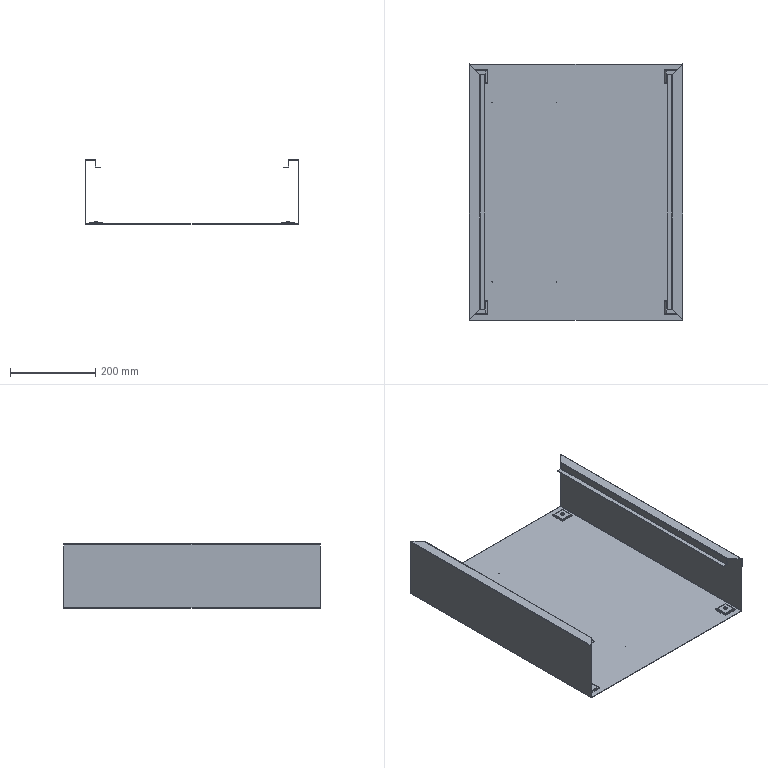Part | SolidWorks | features EdgeFlange 7, LPattern 3, FormToolInstance 2, FlatPattern 1, ICE 1, SMBaseFlange 1, SheetMetal 1 | 1 solid | 224 faces | box 500 x 600 x 150 mm | volume 642827 mm3 | cylinder 114 | plane 106 | spline 4 | commonest cylinder face diameters 1.6 x26 1 x16 3.4 x16 4 x16 5.2 x16 0.4 x8